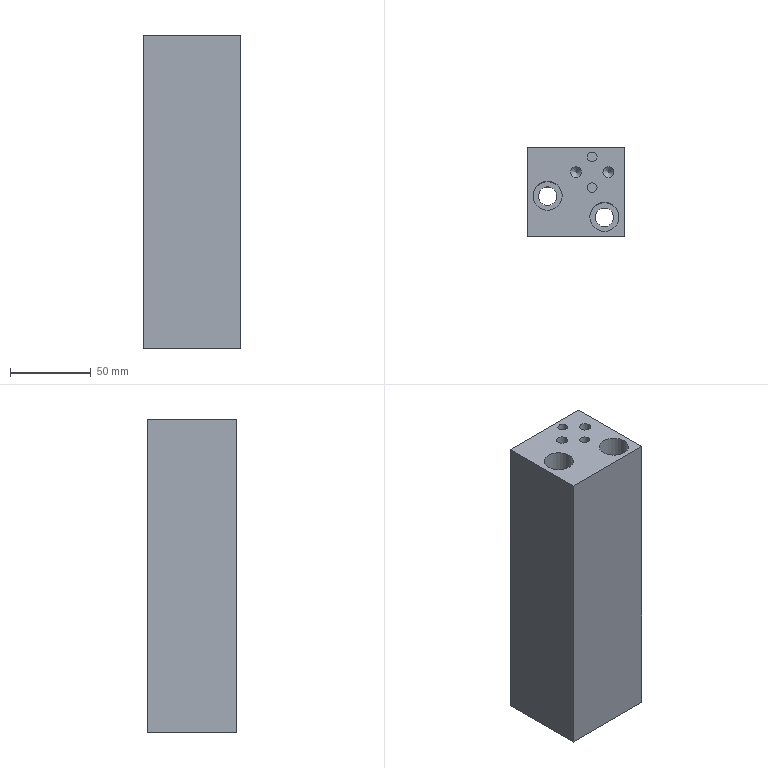Part | NX | features solid 2 | 1 solid | 20 faces | box 60 x 55 x 193.5 mm | volume 545751 mm3 | plane 10 | cylinder 8 | cone 2 | commonest cylinder face diameters 6.001 x2 6.8 x2 11.5 x2 18 x2
STEP:
#1=CARTESIAN_POINT('',(3968.001,-469.5,45.5));
#2=VERTEX_POINT('',#1);
#3=CARTESIAN_POINT('',(3965.,-469.5,45.5));
#4=DIRECTION('',(0.,0.,-1.));
#5=DIRECTION('',(1.,0.,0.));
#6=AXIS2_PLACEMENT_3D('',#3,#4,#5);
#7=CIRCLE('',#6,3.001);
#8=EDGE_CURVE('',#2,#2,#7,.T.);
#9=ORIENTED_EDGE('',*,*,#8,.F.);
#10=EDGE_LOOP('',(#9));
#11=FACE_BOUND('',#10,.T.);
#12=CARTESIAN_POINT('',(3965.,-469.5,45.5));
#13=DIRECTION('',(0.,0.,-1.));
#14=DIRECTION('',(1.,0.,0.));
#15=AXIS2_PLACEMENT_3D('',#12,#13,#14);
#16=PLANE('',#15);
#17=ADVANCED_FACE('',(#11),#16,.F.);
#18=CARTESIAN_POINT('',(3968.001,-488.5,45.5));
#19=VERTEX_POINT('',#18);
#20=CARTESIAN_POINT('',(3965.,-488.5,45.5));
#21=DIRECTION('',(0.,0.,-1.));
#22=DIRECTION('',(1.,0.,0.));
#23=AXIS2_PLACEMENT_3D('',#20,#21,#22);
#24=CIRCLE('',#23,3.001);
#25=EDGE_CURVE('',#19,#19,#24,.T.);
#26=ORIENTED_EDGE('',*,*,#25,.F.);
#27=EDGE_LOOP('',(#26));
#28=FACE_BOUND('',#27,.T.);
#29=CARTESIAN_POINT('',(3965.,-488.5,45.5));
#30=DIRECTION('',(0.,0.,-1.));
#31=DIRECTION('',(1.,0.,0.));
#32=AXIS2_PLACEMENT_3D('',#29,#30,#31);
#33=PLANE('',#32);
#34=ADVANCED_FACE('',(#28),#33,.F.);
#35=CARTESIAN_POINT('',(3968.001,-488.5,70.5));
#36=VERTEX_POINT('',#35);
#37=CARTESIAN_POINT('',(3965.,-488.5,70.5));
#38=DIRECTION('',(0.,0.,-1.));
#39=DIRECTION('',(1.,0.,0.));
#40=AXIS2_PLACEMENT_3D('',#37,#38,#39);
#41=CIRCLE('',#40,3.001);
#42=EDGE_CURVE('',#36,#36,#41,.T.);
#43=ORIENTED_EDGE('',*,*,#42,.T.);
#44=EDGE_LOOP('',(#43));
#45=FACE_BOUND('',#44,.T.);
#46=CARTESIAN_POINT('',(3968.001,-469.5,70.5));
#47=VERTEX_POINT('',#46);
#48=CARTESIAN_POINT('',(3965.,-469.5,70.5));
#49=DIRECTION('',(0.,0.,-1.));
#50=DIRECTION('',(1.,0.,0.));
#51=AXIS2_PLACEMENT_3D('',#48,#49,#50);
#52=CIRCLE('',#51,3.001);
#53=EDGE_CURVE('',#47,#47,#52,.T.);
#54=ORIENTED_EDGE('',*,*,#53,.T.);
#55=EDGE_LOOP('',(#54));
#56=FACE_BOUND('',#55,.T.);
#57=CARTESIAN_POINT('',(3978.4,-479.,70.5));
#58=VERTEX_POINT('',#57);
#59=CARTESIAN_POINT('',(3975.,-479.,70.5));
#60=DIRECTION('',(0.,0.,-1.));
#61=DIRECTION('',(1.,0.,0.));
#62=AXIS2_PLACEMENT_3D('',#59,#60,#61);
#63=CIRCLE('',#62,3.4);
#64=EDGE_CURVE('',#58,#58,#63,.T.);
#65=ORIENTED_EDGE('',*,*,#64,.T.);
#66=EDGE_LOOP('',(#65));
#67=FACE_BOUND('',#66,.T.);
#68=CARTESIAN_POINT('',(3958.4,-479.,70.5));
#69=VERTEX_POINT('',#68);
#70=CARTESIAN_POINT('',(3955.,-479.,70.5));
#71=DIRECTION('',(0.,0.,-1.));
#72=DIRECTION('',(1.,0.,0.));
#73=AXIS2_PLACEMENT_3D('',#70,#71,#72);
#74=CIRCLE('',#73,3.4);
#75=EDGE_CURVE('',#69,#69,#74,.T.);
#76=ORIENTED_EDGE('',*,*,#75,.T.);
#77=EDGE_LOOP('',(#76));
#78=FACE_BOUND('',#77,.T.);
#79=CARTESIAN_POINT('',(3985.,-463.5,70.5));
#80=VERTEX_POINT('',#79);
#81=CARTESIAN_POINT('',(3985.,-518.5,70.5));
#82=VERTEX_POINT('',#81);
#83=CARTESIAN_POINT('',(3985.,-420.,70.5));
#84=DIRECTION('',(0.,-1.,0.));
#85=VECTOR('',#84,1000.);
#86=LINE('',#83,#85);
#87=EDGE_CURVE('',#80,#82,#86,.T.);
#88=ORIENTED_EDGE('',*,*,#87,.F.);
#89=CARTESIAN_POINT('',(3925.,-463.5,70.5));
#90=VERTEX_POINT('',#89);
#91=CARTESIAN_POINT('',(3982.5,-463.5,70.5));
#92=DIRECTION('',(1.,0.,0.));
#93=VECTOR('',#92,1000.);
#94=LINE('',#91,#93);
#95=EDGE_CURVE('',#90,#80,#94,.T.);
#96=ORIENTED_EDGE('',*,*,#95,.F.);
#97=CARTESIAN_POINT('',(3925.,-518.5,70.5));
#98=VERTEX_POINT('',#97);
#99=CARTESIAN_POINT('',(3925.,-602.5,70.5));
#100=DIRECTION('',(0.,-1.,0.));
#101=VECTOR('',#100,1000.);
#102=LINE('',#99,#101);
#103=EDGE_CURVE('',#90,#98,#102,.T.);
#104=ORIENTED_EDGE('',*,*,#103,.T.);
#105=CARTESIAN_POINT('',(3982.5,-518.5,70.5));
#106=DIRECTION('',(-1.,0.,0.));
#107=VECTOR('',#106,1000.);
#108=LINE('',#105,#107);
#109=EDGE_CURVE('',#82,#98,#108,.T.);
#110=ORIENTED_EDGE('',*,*,#109,.F.);
#111=EDGE_LOOP('',(#88,#96,#104,#110));
#112=FACE_BOUND('',#111,.T.);
#113=CARTESIAN_POINT('',(3946.5,-493.5,70.5));
#114=VERTEX_POINT('',#113);
#115=CARTESIAN_POINT('',(3937.5,-493.5,70.5));
#116=DIRECTION('',(0.,0.,-1.));
#117=DIRECTION('',(1.,0.,0.));
#118=AXIS2_PLACEMENT_3D('',#115,#116,#117);
#119=CIRCLE('',#118,9.);
#120=EDGE_CURVE('',#114,#114,#119,.T.);
#121=ORIENTED_EDGE('',*,*,#120,.T.);
#122=EDGE_LOOP('',(#121));
#123=FACE_BOUND('',#122,.T.);
#124=CARTESIAN_POINT('',(3963.5,-506.5,70.5));
#125=VERTEX_POINT('',#124);
#126=CARTESIAN_POINT('',(3972.5,-506.5,70.5));
#127=DIRECTION('',(0.,0.,1.));
#128=DIRECTION('',(-1.,0.,0.));
#129=AXIS2_PLACEMENT_3D('',#126,#127,#128);
#130=CIRCLE('',#129,9.);
#131=EDGE_CURVE('',#125,#125,#130,.T.);
#132=ORIENTED_EDGE('',*,*,#131,.F.);
#133=EDGE_LOOP('',(#132));
#134=FACE_BOUND('',#133,.T.);
#135=CARTESIAN_POINT('',(3982.5,-420.,70.5));
#136=DIRECTION('',(0.,0.,-1.));
#137=DIRECTION('',(0.,1.,0.));
#138=AXIS2_PLACEMENT_3D('',#135,#136,#137);
#139=PLANE('',#138);
#140=ADVANCED_FACE('',(#45,#56,#67,#78,#112,#123,#134),#139,.F.);
#141=CARTESIAN_POINT('',(3966.75,-506.5,-123.));
#142=VERTEX_POINT('',#141);
#143=CARTESIAN_POINT('',(3972.5,-506.5,-123.));
#144=DIRECTION('',(0.,0.,-1.));
#145=DIRECTION('',(-1.,0.,0.));
#146=AXIS2_PLACEMENT_3D('',#143,#144,#145);
#147=CIRCLE('',#146,5.75);
#148=EDGE_CURVE('',#142,#142,#147,.T.);
#149=ORIENTED_EDGE('',*,*,#148,.F.);
#150=EDGE_LOOP('',(#149));
#151=FACE_BOUND('',#150,.T.);
#152=CARTESIAN_POINT('',(3985.,-518.5,-123.));
#153=VERTEX_POINT('',#152);
#154=CARTESIAN_POINT('',(3985.,-463.5,-123.));
#155=VERTEX_POINT('',#154);
#156=CARTESIAN_POINT('',(3985.,-481.,-123.));
#157=DIRECTION('',(0.,1.,0.));
#158=VECTOR('',#157,1000.);
#159=LINE('',#156,#158);
#160=EDGE_CURVE('',#153,#155,#159,.T.);
#161=ORIENTED_EDGE('',*,*,#160,.F.);
#162=CARTESIAN_POINT('',(3925.,-518.5,-123.));
#163=VERTEX_POINT('',#162);
#164=CARTESIAN_POINT('',(3982.5,-518.5,-123.));
#165=DIRECTION('',(1.,0.,0.));
#166=VECTOR('',#165,1000.);
#167=LINE('',#164,#166);
#168=EDGE_CURVE('',#163,#153,#167,.T.);
#169=ORIENTED_EDGE('',*,*,#168,.F.);
#170=CARTESIAN_POINT('',(3925.,-463.5,-123.));
#171=VERTEX_POINT('',#170);
#172=CARTESIAN_POINT('',(3925.,-602.5,-123.));
#173=DIRECTION('',(0.,-1.,0.));
#174=VECTOR('',#173,1000.);
#175=LINE('',#172,#174);
#176=EDGE_CURVE('',#171,#163,#175,.T.);
#177=ORIENTED_EDGE('',*,*,#176,.F.);
#178=CARTESIAN_POINT('',(3982.5,-463.5,-123.));
#179=DIRECTION('',(-1.,0.,0.));
#180=VECTOR('',#179,1000.);
#181=LINE('',#178,#180);
#182=EDGE_CURVE('',#155,#171,#181,.T.);
#183=ORIENTED_EDGE('',*,*,#182,.F.);
#184=EDGE_LOOP('',(#161,#169,#177,#183));
#185=FACE_BOUND('',#184,.T.);
#186=CARTESIAN_POINT('',(3943.25,-493.5,-123.));
#187=VERTEX_POINT('',#186);
#188=CARTESIAN_POINT('',(3937.5,-493.5,-123.));
#189=DIRECTION('',(0.,0.,1.));
#190=DIRECTION('',(1.,0.,0.));
#191=AXIS2_PLACEMENT_3D('',#188,#189,#190);
#192=CIRCLE('',#191,5.75);
#193=EDGE_CURVE('',#187,#187,#192,.T.);
#194=ORIENTED_EDGE('',*,*,#193,.T.);
#195=EDGE_LOOP('',(#194));
#196=FACE_BOUND('',#195,.T.);
#197=CARTESIAN_POINT('',(3427.5,0.,-123.));
#198=DIRECTION('',(0.,0.,-1.));
#199=DIRECTION('',(1.,0.,0.));
#200=AXIS2_PLACEMENT_3D('',#197,#198,#199);
#201=PLANE('',#200);
#202=ADVANCED_FACE('',(#151,#185,#196),#201,.T.);
#203=CARTESIAN_POINT('',(3925.,-518.5,28.));
#204=DIRECTION('',(0.,0.,-1.));
#205=VECTOR('',#204,1000.);
#206=LINE('',#203,#205);
#207=EDGE_CURVE('',#98,#163,#206,.T.);
#208=ORIENTED_EDGE('',*,*,#207,.T.);
#209=ORIENTED_EDGE('',*,*,#168,.T.);
#210=CARTESIAN_POINT('',(3985.,-518.5,46.5));
#211=DIRECTION('',(0.,0.,-1.));
#212=VECTOR('',#211,1000.);
#213=LINE('',#210,#212);
#214=EDGE_CURVE('',#82,#153,#213,.T.);
#215=ORIENTED_EDGE('',*,*,#214,.F.);
#216=ORIENTED_EDGE('',*,*,#109,.T.);
#217=EDGE_LOOP('',(#208,#209,#215,#216));
#218=FACE_BOUND('',#217,.T.);
#219=CARTESIAN_POINT('',(3982.5,-518.5,28.));
#220=DIRECTION('',(0.,-1.,0.));
#221=DIRECTION('',(0.,0.,-1.));
#222=AXIS2_PLACEMENT_3D('',#219,#220,#221);
#223=PLANE('',#222);
#224=ADVANCED_FACE('',(#218),#223,.T.);
#225=CARTESIAN_POINT('',(3985.,-463.5,46.5));
#226=DIRECTION('',(0.,0.,1.));
#227=VECTOR('',#226,1000.);
#228=LINE('',#225,#227);
#229=EDGE_CURVE('',#155,#80,#228,.T.);
#230=ORIENTED_EDGE('',*,*,#229,.F.);
#231=ORIENTED_EDGE('',*,*,#182,.T.);
#232=CARTESIAN_POINT('',(3925.,-463.5,28.));
#233=DIRECTION('',(0.,0.,1.));
#234=VECTOR('',#233,1000.);
#235=LINE('',#232,#234);
#236=EDGE_CURVE('',#171,#90,#235,.T.);
#237=ORIENTED_EDGE('',*,*,#236,.T.);
#238=ORIENTED_EDGE('',*,*,#95,.T.);
#239=EDGE_LOOP('',(#230,#231,#237,#238));
#240=FACE_BOUND('',#239,.T.);
#241=CARTESIAN_POINT('',(3982.5,-463.5,28.));
#242=DIRECTION('',(0.,1.,0.));
#243=DIRECTION('',(0.,0.,1.));
#244=AXIS2_PLACEMENT_3D('',#241,#242,#243);
#245=PLANE('',#244);
#246=ADVANCED_FACE('',(#240),#245,.T.);
#247=ORIENTED_EDGE('',*,*,#214,.T.);
#248=ORIENTED_EDGE('',*,*,#160,.T.);
#249=ORIENTED_EDGE('',*,*,#229,.T.);
#250=ORIENTED_EDGE('',*,*,#87,.T.);
#251=EDGE_LOOP('',(#247,#248,#249,#250));
#252=FACE_BOUND('',#251,.T.);
#253=CARTESIAN_POINT('',(3985.,-481.,46.5));
#254=DIRECTION('',(1.,0.,0.));
#255=DIRECTION('',(0.,1.,0.));
#256=AXIS2_PLACEMENT_3D('',#253,#254,#255);
#257=PLANE('',#256);
#258=ADVANCED_FACE('',(#252),#257,.T.);
#259=ORIENTED_EDGE('',*,*,#236,.F.);
#260=ORIENTED_EDGE('',*,*,#176,.T.);
#261=ORIENTED_EDGE('',*,*,#207,.F.);
#262=ORIENTED_EDGE('',*,*,#103,.F.);
#263=EDGE_LOOP('',(#259,#260,#261,#262));
#264=FACE_BOUND('',#263,.T.);
#265=CARTESIAN_POINT('',(3925.,-602.5,-113.));
#266=DIRECTION('',(-1.,0.,0.));
#267=DIRECTION('',(0.,0.,-1.));
#268=AXIS2_PLACEMENT_3D('',#265,#266,#267);
#269=PLANE('',#268);
#270=ADVANCED_FACE('',(#264),#269,.T.);
#271=CARTESIAN_POINT('',(3931.75,-493.5,-93.));
#272=VERTEX_POINT('',#271);
#273=CARTESIAN_POINT('',(3937.5,-493.5,-93.));
#274=DIRECTION('',(0.,0.,-1.));
#275=DIRECTION('',(-1.,0.,0.));
#276=AXIS2_PLACEMENT_3D('',#273,#274,#275);
#277=CIRCLE('',#276,5.75);
#278=EDGE_CURVE('',#272,#272,#277,.T.);
#279=ORIENTED_EDGE('',*,*,#278,.F.);
#280=EDGE_LOOP('',(#279));
#281=FACE_BOUND('',#280,.T.);
#282=ORIENTED_EDGE('',*,*,#193,.F.);
#283=EDGE_LOOP('',(#282));
#284=FACE_BOUND('',#283,.T.);
#285=CARTESIAN_POINT('',(3937.5,-493.5,70.5));
#286=DIRECTION('',(0.,0.,-1.));
#287=DIRECTION('',(-1.,0.,0.));
#288=AXIS2_PLACEMENT_3D('',#285,#286,#287);
#289=CYLINDRICAL_SURFACE('',#288,5.75);
#290=ADVANCED_FACE('',(#281,#284),#289,.F.);
#291=ORIENTED_EDGE('',*,*,#278,.T.);
#292=EDGE_LOOP('',(#291));
#293=FACE_BOUND('',#292,.T.);
#294=CARTESIAN_POINT('',(3928.5,-493.5,-93.));
#295=VERTEX_POINT('',#294);
#296=CARTESIAN_POINT('',(3937.5,-493.5,-93.));
#297=DIRECTION('',(0.,0.,-1.));
#298=DIRECTION('',(-1.,0.,0.));
#299=AXIS2_PLACEMENT_3D('',#296,#297,#298);
#300=CIRCLE('',#299,9.);
#301=EDGE_CURVE('',#295,#295,#300,.T.);
#302=ORIENTED_EDGE('',*,*,#301,.F.);
#303=EDGE_LOOP('',(#302));
#304=FACE_BOUND('',#303,.T.);
#305=CARTESIAN_POINT('',(3427.5,0.,-93.));
#306=DIRECTION('',(0.,0.,-1.));
#307=DIRECTION('',(1.,0.,0.));
#308=AXIS2_PLACEMENT_3D('',#305,#306,#307);
#309=PLANE('',#308);
#310=ADVANCED_FACE('',(#293,#304),#309,.F.);
#311=ORIENTED_EDGE('',*,*,#301,.T.);
#312=EDGE_LOOP('',(#311));
#313=FACE_BOUND('',#312,.T.);
#314=ORIENTED_EDGE('',*,*,#120,.F.);
#315=EDGE_LOOP('',(#314));
#316=FACE_BOUND('',#315,.T.);
#317=CARTESIAN_POINT('',(3937.5,-493.5,70.5));
#318=DIRECTION('',(0.,0.,-1.));
#319=DIRECTION('',(-1.,0.,0.));
#320=AXIS2_PLACEMENT_3D('',#317,#318,#319);
#321=CYLINDRICAL_SURFACE('',#320,9.);
#322=ADVANCED_FACE('',(#313,#316),#321,.F.);
#323=CARTESIAN_POINT('',(3966.75,-506.5,-93.));
#324=VERTEX_POINT('',#323);
#325=CARTESIAN_POINT('',(3972.5,-506.5,-93.));
#326=DIRECTION('',(0.,0.,1.));
#327=DIRECTION('',(-1.,0.,0.));
#328=AXIS2_PLACEMENT_3D('',#325,#326,#327);
#329=CIRCLE('',#328,5.75);
#330=EDGE_CURVE('',#324,#324,#329,.T.);
#331=ORIENTED_EDGE('',*,*,#330,.T.);
#332=EDGE_LOOP('',(#331));
#333=FACE_BOUND('',#332,.T.);
#334=ORIENTED_EDGE('',*,*,#148,.T.);
#335=EDGE_LOOP('',(#334));
#336=FACE_BOUND('',#335,.T.);
#337=CARTESIAN_POINT('',(3972.5,-506.5,70.5));
#338=DIRECTION('',(0.,0.,-1.));
#339=DIRECTION('',(1.,0.,0.));
#340=AXIS2_PLACEMENT_3D('',#337,#338,#339);
#341=CYLINDRICAL_SURFACE('',#340,5.75);
#342=ADVANCED_FACE('',(#333,#336),#341,.F.);
#343=ORIENTED_EDGE('',*,*,#330,.F.);
#344=EDGE_LOOP('',(#343));
#345=FACE_BOUND('',#344,.T.);
#346=CARTESIAN_POINT('',(3963.5,-506.5,-93.));
#347=VERTEX_POINT('',#346);
#348=CARTESIAN_POINT('',(3972.5,-506.5,-93.));
#349=DIRECTION('',(0.,0.,1.));
#350=DIRECTION('',(-1.,0.,0.));
#351=AXIS2_PLACEMENT_3D('',#348,#349,#350);
#352=CIRCLE('',#351,9.);
#353=EDGE_CURVE('',#347,#347,#352,.T.);
#354=ORIENTED_EDGE('',*,*,#353,.T.);
#355=EDGE_LOOP('',(#354));
#356=FACE_BOUND('',#355,.T.);
#357=CARTESIAN_POINT('',(3427.5,0.,-93.));
#358=DIRECTION('',(0.,0.,-1.));
#359=DIRECTION('',(1.,0.,0.));
#360=AXIS2_PLACEMENT_3D('',#357,#358,#359);
#361=PLANE('',#360);
#362=ADVANCED_FACE('',(#345,#356),#361,.F.);
#363=ORIENTED_EDGE('',*,*,#353,.F.);
#364=EDGE_LOOP('',(#363));
#365=FACE_BOUND('',#364,.T.);
#366=ORIENTED_EDGE('',*,*,#131,.T.);
#367=EDGE_LOOP('',(#366));
#368=FACE_BOUND('',#367,.T.);
#369=CARTESIAN_POINT('',(3972.5,-506.5,70.5));
#370=DIRECTION('',(0.,0.,-1.));
#371=DIRECTION('',(1.,0.,0.));
#372=AXIS2_PLACEMENT_3D('',#369,#370,#371);
#373=CYLINDRICAL_SURFACE('',#372,9.);
#374=ADVANCED_FACE('',(#365,#368),#373,.F.);
#375=CARTESIAN_POINT('',(3951.6,-479.,44.9));
#376=VERTEX_POINT('',#375);
#377=CARTESIAN_POINT('',(3955.,-479.,44.9));
#378=DIRECTION('',(0.,0.,-1.));
#379=DIRECTION('',(-1.,0.,0.));
#380=AXIS2_PLACEMENT_3D('',#377,#378,#379);
#381=CIRCLE('',#380,3.4);
#382=EDGE_CURVE('',#376,#376,#381,.T.);
#383=ORIENTED_EDGE('',*,*,#382,.T.);
#384=EDGE_LOOP('',(#383));
#385=FACE_BOUND('',#384,.T.);
#386=ORIENTED_EDGE('',*,*,#75,.F.);
#387=EDGE_LOOP('',(#386));
#388=FACE_BOUND('',#387,.T.);
#389=CARTESIAN_POINT('',(3955.,-479.,70.5));
#390=DIRECTION('',(0.,0.,-1.));
#391=DIRECTION('',(-1.,0.,0.));
#392=AXIS2_PLACEMENT_3D('',#389,#390,#391);
#393=CYLINDRICAL_SURFACE('',#392,3.4);
#394=ADVANCED_FACE('',(#385,#388),#393,.F.);
#395=CARTESIAN_POINT('',(3955.,-479.,41.5));
#396=VERTEX_POINT('',#395);
#397=VERTEX_LOOP('',#396);
#398=FACE_BOUND('',#397,.T.);
#399=ORIENTED_EDGE('',*,*,#382,.F.);
#400=EDGE_LOOP('',(#399));
#401=FACE_BOUND('',#400,.T.);
#402=CARTESIAN_POINT('',(3955.,-479.,44.9));
#403=DIRECTION('',(0.,0.,1.));
#404=DIRECTION('',(-1.,0.,0.));
#405=AXIS2_PLACEMENT_3D('',#402,#403,#404);
#406=CONICAL_SURFACE('',#405,3.4,0.7854);
#407=ADVANCED_FACE('',(#398,#401),#406,.F.);
#408=CARTESIAN_POINT('',(3971.6,-479.,44.9));
#409=VERTEX_POINT('',#408);
#410=CARTESIAN_POINT('',(3975.,-479.,44.9));
#411=DIRECTION('',(0.,0.,-1.));
#412=DIRECTION('',(-1.,0.,0.));
#413=AXIS2_PLACEMENT_3D('',#410,#411,#412);
#414=CIRCLE('',#413,3.4);
#415=EDGE_CURVE('',#409,#409,#414,.T.);
#416=ORIENTED_EDGE('',*,*,#415,.T.);
#417=EDGE_LOOP('',(#416));
#418=FACE_BOUND('',#417,.T.);
#419=ORIENTED_EDGE('',*,*,#64,.F.);
#420=EDGE_LOOP('',(#419));
#421=FACE_BOUND('',#420,.T.);
#422=CARTESIAN_POINT('',(3975.,-479.,70.5));
#423=DIRECTION('',(0.,0.,-1.));
#424=DIRECTION('',(-1.,0.,0.));
#425=AXIS2_PLACEMENT_3D('',#422,#423,#424);
#426=CYLINDRICAL_SURFACE('',#425,3.4);
#427=ADVANCED_FACE('',(#418,#421),#426,.F.);
#428=CARTESIAN_POINT('',(3975.,-479.,41.5));
#429=VERTEX_POINT('',#428);
#430=VERTEX_LOOP('',#429);
#431=FACE_BOUND('',#430,.T.);
#432=ORIENTED_EDGE('',*,*,#415,.F.);
#433=EDGE_LOOP('',(#432));
#434=FACE_BOUND('',#433,.T.);
#435=CARTESIAN_POINT('',(3975.,-479.,44.9));
#436=DIRECTION('',(0.,0.,1.));
#437=DIRECTION('',(-1.,0.,0.));
#438=AXIS2_PLACEMENT_3D('',#435,#436,#437);
#439=CONICAL_SURFACE('',#438,3.4,0.7854);
#440=ADVANCED_FACE('',(#431,#434),#439,.F.);
#441=ORIENTED_EDGE('',*,*,#8,.T.);
#442=EDGE_LOOP('',(#441));
#443=FACE_BOUND('',#442,.T.);
#444=ORIENTED_EDGE('',*,*,#53,.F.);
#445=EDGE_LOOP('',(#444));
#446=FACE_BOUND('',#445,.T.);
#447=CARTESIAN_POINT('',(3965.,-469.5,70.5));
#448=DIRECTION('',(0.,0.,-1.));
#449=DIRECTION('',(-1.,0.,0.));
#450=AXIS2_PLACEMENT_3D('',#447,#448,#449);
#451=CYLINDRICAL_SURFACE('',#450,3.001);
#452=ADVANCED_FACE('',(#443,#446),#451,.F.);
#453=ORIENTED_EDGE('',*,*,#25,.T.);
#454=EDGE_LOOP('',(#453));
#455=FACE_BOUND('',#454,.T.);
#456=ORIENTED_EDGE('',*,*,#42,.F.);
#457=EDGE_LOOP('',(#456));
#458=FACE_BOUND('',#457,.T.);
#459=CARTESIAN_POINT('',(3965.,-488.5,70.5));
#460=DIRECTION('',(0.,0.,-1.));
#461=DIRECTION('',(-1.,0.,0.));
#462=AXIS2_PLACEMENT_3D('',#459,#460,#461);
#463=CYLINDRICAL_SURFACE('',#462,3.001);
#464=ADVANCED_FACE('',(#455,#458),#463,.F.);
#465=CLOSED_SHELL('',(#17,#34,#140,#202,#224,#246,#258,#270,#290,#310,#322,#342,#362,#374,#394,#407,#427,#440,#452,#464));
#466=MANIFOLD_SOLID_BREP('',#465);
#467=(LENGTH_UNIT()NAMED_UNIT(*)SI_UNIT(.MILLI.,.METRE.));
#468=UNCERTAINTY_MEASURE_WITH_UNIT(LENGTH_MEASURE(0.00001),#467,'','');
#469=(NAMED_UNIT(*)PLANE_ANGLE_UNIT()SI_UNIT($,.RADIAN.));
#470=(NAMED_UNIT(*)SI_UNIT($,.STERADIAN.)SOLID_ANGLE_UNIT());
#471=(GEOMETRIC_REPRESENTATION_CONTEXT(3)GLOBAL_UNCERTAINTY_ASSIGNED_CONTEXT((#468))GLOBAL_UNIT_ASSIGNED_CONTEXT((#467,#469,#470))REPRESENTATION_CONTEXT('',''));
#472=ADVANCED_BREP_SHAPE_REPRESENTATION('',(#466),#471);